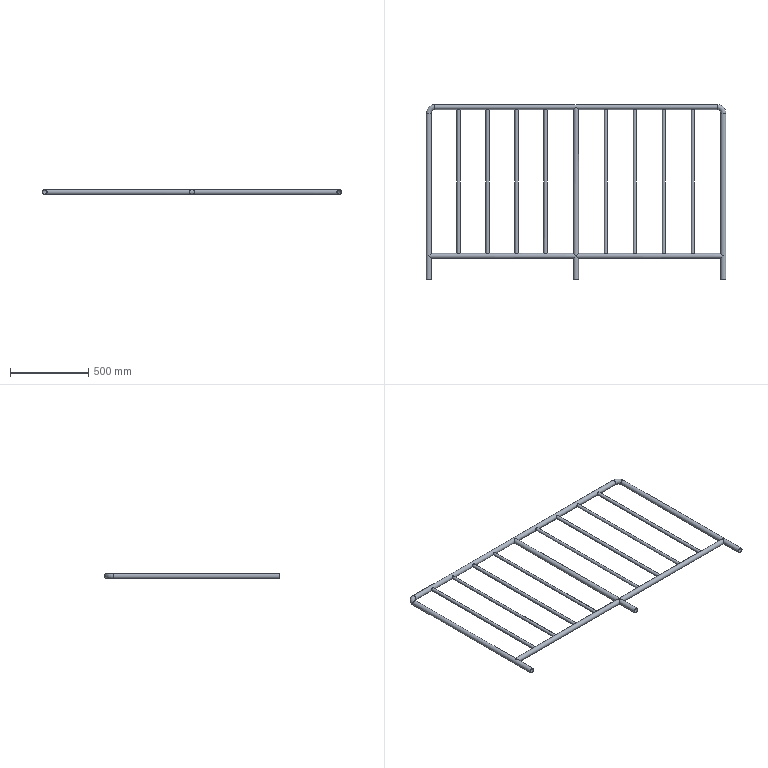Part | STEP file | 304 guardrail 1880X1100 body_Default<As Machined> | 16 solids | 64 faces | box 1912 x 1116 x 32 mm | volume 1441532 mm3 | cylinder 49 | plane 11 | torus 4 | commonest cylinder face diameters 32 x27 18 x8 20 x8 29 x6